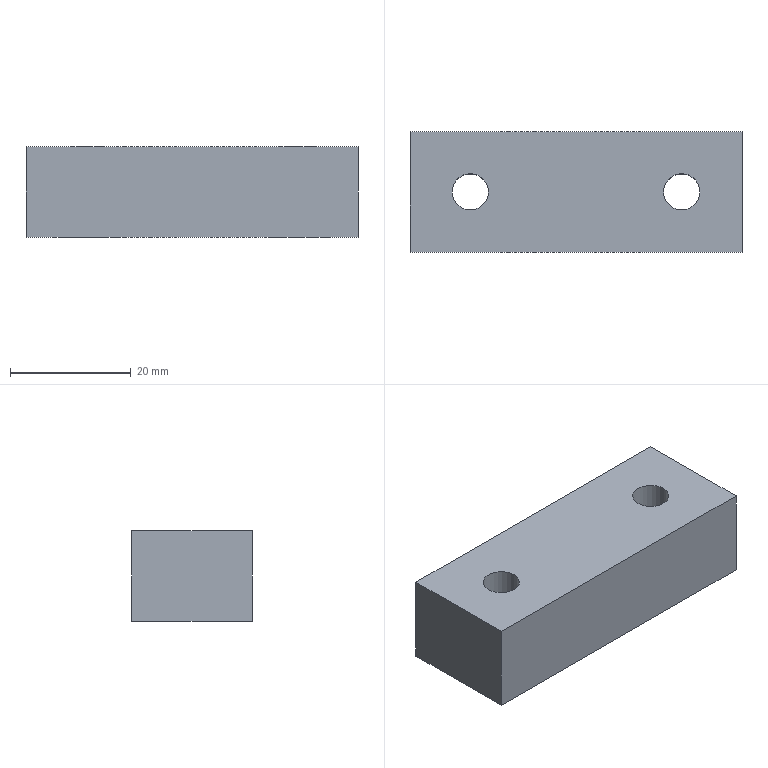Part | STEP file | gslz 2016.10.28-10_id2086_x_t | 1 solid | 12 faces | box 55 x 20 x 15 mm | volume 14584 mm3 | plane 8 | cylinder 4 | commonest cylinder face diameters 6 x2 11 x2
STEP:
#1=CARTESIAN_POINT('',(0.,0.,0.));
#2=DIRECTION('',(0.,0.,1.));
#3=DIRECTION('',(1.,0.,0.));
#4=AXIS2_PLACEMENT_3D('',#1,#2,#3);
#5=CARTESIAN_POINT('',(353.5,240.,28.));
#6=VERTEX_POINT('',#5);
#7=CARTESIAN_POINT('',(359.,240.,28.));
#8=DIRECTION('',(0.,0.,1.));
#9=DIRECTION('',(-1.,0.,0.));
#10=AXIS2_PLACEMENT_3D('',#7,#8,#9);
#11=CIRCLE('',#10,5.5);
#12=CARTESIAN_POINT('',(359.,240.,30.));
#13=DIRECTION('',(0.,0.,-1.));
#14=DIRECTION('',(-1.,0.,0.));
#15=AXIS2_PLACEMENT_3D('',#12,#13,#14);
#16=CYLINDRICAL_SURFACE('',#15,5.5);
#17=CARTESIAN_POINT('',(6.283,2.));
#18=DIRECTION('',(-1.,0.));
#19=VECTOR('',#18,1.);
#20=LINE('',#17,#19);
#21=(GEOMETRIC_REPRESENTATION_CONTEXT(2)PARAMETRIC_REPRESENTATION_CONTEXT()REPRESENTATION_CONTEXT('',''));
#22=DEFINITIONAL_REPRESENTATION('',(#20),#21);
#23=PCURVE('',#16,#22);
#24=CARTESIAN_POINT('',(396.5,240.,28.));
#25=DIRECTION('',(0.,0.,-1.));
#26=DIRECTION('',(1.,0.,0.));
#27=AXIS2_PLACEMENT_3D('',#24,#25,#26);
#28=PLANE('',#27);
#29=CARTESIAN_POINT('',(-43.,0.));
#30=CARTESIAN_POINT('',(-43.,9.526));
#31=CARTESIAN_POINT('',(-34.75,4.763));
#32=CARTESIAN_POINT('',(-26.5,0.));
#33=CARTESIAN_POINT('',(-34.75,-4.763));
#34=CARTESIAN_POINT('',(-43.,-9.526));
#35=CARTESIAN_POINT('',(-43.,0.));
#36=(BOUNDED_CURVE()B_SPLINE_CURVE(2,(#29,#30,#31,#32,#33,#34,#35),.UNSPECIFIED.,.T.,.F.)B_SPLINE_CURVE_WITH_KNOTS((1,2,2,2,2,1),(-2.094,0.,2.094,4.189,6.283,8.378),.UNSPECIFIED.)CURVE()GEOMETRIC_REPRESENTATION_ITEM()RATIONAL_B_SPLINE_CURVE((1.,0.5,1.,0.5,1.,0.5,1.))REPRESENTATION_ITEM(''));
#37=(GEOMETRIC_REPRESENTATION_CONTEXT(2)PARAMETRIC_REPRESENTATION_CONTEXT()REPRESENTATION_CONTEXT('',''));
#38=DEFINITIONAL_REPRESENTATION('',(#36),#37);
#39=PCURVE('',#28,#38);
#40=SURFACE_CURVE('',#11,(#23,#39),.PCURVE_S1.);
#41=EDGE_CURVE('',#6,#6,#40,.T.);
#42=ORIENTED_EDGE('',*,*,#41,.F.);
#43=CARTESIAN_POINT('',(353.5,240.,20.));
#44=VERTEX_POINT('',#43);
#45=CARTESIAN_POINT('',(353.5,240.,28.));
#46=CARTESIAN_POINT('',(353.5,240.,20.));
#47=B_SPLINE_CURVE_WITH_KNOTS('',1,(#45,#46),.UNSPECIFIED.,.F.,.F.,(2,2),(2.,10.),.PIECEWISE_BEZIER_KNOTS.);
#48=CARTESIAN_POINT('',(6.283,0.));
#49=DIRECTION('',(0.,1.));
#50=VECTOR('',#49,1.);
#51=LINE('',#48,#50);
#52=(GEOMETRIC_REPRESENTATION_CONTEXT(2)PARAMETRIC_REPRESENTATION_CONTEXT()REPRESENTATION_CONTEXT('',''));
#53=DEFINITIONAL_REPRESENTATION('',(#51),#52);
#54=PCURVE('',#16,#53);
#55=CARTESIAN_POINT('',(0.,0.));
#56=DIRECTION('',(0.,1.));
#57=VECTOR('',#56,1.);
#58=LINE('',#55,#57);
#59=(GEOMETRIC_REPRESENTATION_CONTEXT(2)PARAMETRIC_REPRESENTATION_CONTEXT()REPRESENTATION_CONTEXT('',''));
#60=DEFINITIONAL_REPRESENTATION('',(#58),#59);
#61=PCURVE('',#16,#60);
#62=SEAM_CURVE('',#47,(#54,#61),.PCURVE_S1.);
#63=EDGE_CURVE('',#6,#44,#62,.T.);
#64=ORIENTED_EDGE('',*,*,#63,.T.);
#65=CARTESIAN_POINT('',(364.5,240.,20.));
#66=VERTEX_POINT('',#65);
#67=CARTESIAN_POINT('',(359.,240.,20.));
#68=DIRECTION('',(0.,0.,1.));
#69=DIRECTION('',(1.,0.,0.));
#70=AXIS2_PLACEMENT_3D('',#67,#68,#69);
#71=CIRCLE('',#70,5.5);
#72=CARTESIAN_POINT('',(9.425,10.));
#73=DIRECTION('',(-1.,0.));
#74=VECTOR('',#73,1.);
#75=LINE('',#72,#74);
#76=(GEOMETRIC_REPRESENTATION_CONTEXT(2)PARAMETRIC_REPRESENTATION_CONTEXT()REPRESENTATION_CONTEXT('',''));
#77=DEFINITIONAL_REPRESENTATION('',(#75),#76);
#78=PCURVE('',#16,#77);
#79=CARTESIAN_POINT('',(301.5,240.,20.));
#80=DIRECTION('',(0.,0.,1.));
#81=DIRECTION('',(1.,0.,0.));
#82=AXIS2_PLACEMENT_3D('',#79,#80,#81);
#83=PLANE('',#82);
#84=CARTESIAN_POINT('',(57.5,0.));
#85=DIRECTION('',(1.,0.));
#86=AXIS2_PLACEMENT_2D('',#84,#85);
#87=CIRCLE('',#86,5.5);
#88=(GEOMETRIC_REPRESENTATION_CONTEXT(2)PARAMETRIC_REPRESENTATION_CONTEXT()REPRESENTATION_CONTEXT('',''));
#89=DEFINITIONAL_REPRESENTATION('',(#87),#88);
#90=PCURVE('',#83,#89);
#91=SURFACE_CURVE('',#71,(#78,#90),.PCURVE_S1.);
#92=EDGE_CURVE('',#44,#66,#91,.T.);
#93=ORIENTED_EDGE('',*,*,#92,.T.);
#94=CARTESIAN_POINT('',(359.,240.,20.));
#95=DIRECTION('',(0.,0.,1.));
#96=DIRECTION('',(1.,0.,0.));
#97=AXIS2_PLACEMENT_3D('',#94,#95,#96);
#98=CIRCLE('',#97,5.5);
#99=CARTESIAN_POINT('',(3.142,10.));
#100=DIRECTION('',(-1.,0.));
#101=VECTOR('',#100,1.);
#102=LINE('',#99,#101);
#103=(GEOMETRIC_REPRESENTATION_CONTEXT(2)PARAMETRIC_REPRESENTATION_CONTEXT()REPRESENTATION_CONTEXT('',''));
#104=DEFINITIONAL_REPRESENTATION('',(#102),#103);
#105=PCURVE('',#16,#104);
#106=CARTESIAN_POINT('',(57.5,0.));
#107=DIRECTION('',(1.,0.));
#108=AXIS2_PLACEMENT_2D('',#106,#107);
#109=CIRCLE('',#108,5.5);
#110=(GEOMETRIC_REPRESENTATION_CONTEXT(2)PARAMETRIC_REPRESENTATION_CONTEXT()REPRESENTATION_CONTEXT('',''));
#111=DEFINITIONAL_REPRESENTATION('',(#109),#110);
#112=PCURVE('',#83,#111);
#113=SURFACE_CURVE('',#98,(#105,#112),.PCURVE_S1.);
#114=EDGE_CURVE('',#66,#44,#113,.T.);
#115=ORIENTED_EDGE('',*,*,#114,.T.);
#116=ORIENTED_EDGE('',*,*,#63,.F.);
#117=EDGE_LOOP('',(#42,#64,#93,#115,#116));
#118=FACE_BOUND('',#117,.F.);
#119=ADVANCED_FACE('',(#118),#16,.F.);
#120=CARTESIAN_POINT('',(349.,250.,35.));
#121=VERTEX_POINT('',#120);
#122=CARTESIAN_POINT('',(349.,250.,20.));
#123=VERTEX_POINT('',#122);
#124=CARTESIAN_POINT('',(349.,250.,30.));
#125=DIRECTION('',(0.,0.,-1.));
#126=VECTOR('',#125,1.);
#127=LINE('',#124,#126);
#128=CARTESIAN_POINT('',(421.5,250.,30.));
#129=DIRECTION('',(0.,-1.,0.));
#130=DIRECTION('',(0.,0.,-1.));
#131=AXIS2_PLACEMENT_3D('',#128,#129,#130);
#132=PLANE('',#131);
#133=CARTESIAN_POINT('',(0.,-72.5));
#134=DIRECTION('',(1.,0.));
#135=VECTOR('',#134,1.);
#136=LINE('',#133,#135);
#137=(GEOMETRIC_REPRESENTATION_CONTEXT(2)PARAMETRIC_REPRESENTATION_CONTEXT()REPRESENTATION_CONTEXT('',''));
#138=DEFINITIONAL_REPRESENTATION('',(#136),#137);
#139=PCURVE('',#132,#138);
#140=CARTESIAN_POINT('',(349.,252.5,30.));
#141=DIRECTION('',(1.,0.,0.));
#142=DIRECTION('',(0.,0.,-1.));
#143=AXIS2_PLACEMENT_3D('',#140,#141,#142);
#144=PLANE('',#143);
#145=CARTESIAN_POINT('',(0.,-2.5));
#146=DIRECTION('',(1.,0.));
#147=VECTOR('',#146,1.);
#148=LINE('',#145,#147);
#149=(GEOMETRIC_REPRESENTATION_CONTEXT(2)PARAMETRIC_REPRESENTATION_CONTEXT()REPRESENTATION_CONTEXT('',''));
#150=DEFINITIONAL_REPRESENTATION('',(#148),#149);
#151=PCURVE('',#144,#150);
#152=SURFACE_CURVE('',#127,(#139,#151),.PCURVE_S1.);
#153=EDGE_CURVE('',#121,#123,#152,.T.);
#154=ORIENTED_EDGE('',*,*,#153,.F.);
#155=CARTESIAN_POINT('',(404.,250.,35.));
#156=VERTEX_POINT('',#155);
#157=CARTESIAN_POINT('',(301.5,250.,35.));
#158=DIRECTION('',(-1.,0.,0.));
#159=VECTOR('',#158,1.);
#160=LINE('',#157,#159);
#161=CARTESIAN_POINT('',(-5.,-120.));
#162=DIRECTION('',(0.,-1.));
#163=VECTOR('',#162,1.);
#164=LINE('',#161,#163);
#165=(GEOMETRIC_REPRESENTATION_CONTEXT(2)PARAMETRIC_REPRESENTATION_CONTEXT()REPRESENTATION_CONTEXT('',''));
#166=DEFINITIONAL_REPRESENTATION('',(#164),#165);
#167=PCURVE('',#132,#166);
#168=CARTESIAN_POINT('',(301.5,240.,35.));
#169=DIRECTION('',(0.,0.,1.));
#170=DIRECTION('',(1.,0.,0.));
#171=AXIS2_PLACEMENT_3D('',#168,#169,#170);
#172=PLANE('',#171);
#173=CARTESIAN_POINT('',(0.,10.));
#174=DIRECTION('',(-1.,0.));
#175=VECTOR('',#174,1.);
#176=LINE('',#173,#175);
#177=(GEOMETRIC_REPRESENTATION_CONTEXT(2)PARAMETRIC_REPRESENTATION_CONTEXT()REPRESENTATION_CONTEXT('',''));
#178=DEFINITIONAL_REPRESENTATION('',(#176),#177);
#179=PCURVE('',#172,#178);
#180=SURFACE_CURVE('',#160,(#167,#179),.PCURVE_S1.);
#181=EDGE_CURVE('',#156,#121,#180,.T.);
#182=ORIENTED_EDGE('',*,*,#181,.F.);
#183=CARTESIAN_POINT('',(404.,250.,20.));
#184=VERTEX_POINT('',#183);
#185=CARTESIAN_POINT('',(404.,250.,30.));
#186=DIRECTION('',(0.,0.,-1.));
#187=VECTOR('',#186,1.);
#188=LINE('',#185,#187);
#189=CARTESIAN_POINT('',(0.,-17.5));
#190=DIRECTION('',(1.,0.));
#191=VECTOR('',#190,1.);
#192=LINE('',#189,#191);
#193=(GEOMETRIC_REPRESENTATION_CONTEXT(2)PARAMETRIC_REPRESENTATION_CONTEXT()REPRESENTATION_CONTEXT('',''));
#194=DEFINITIONAL_REPRESENTATION('',(#192),#193);
#195=PCURVE('',#132,#194);
#196=CARTESIAN_POINT('',(404.,227.5,30.));
#197=DIRECTION('',(-1.,0.,0.));
#198=DIRECTION('',(0.,0.,1.));
#199=AXIS2_PLACEMENT_3D('',#196,#197,#198);
#200=PLANE('',#199);
#201=CARTESIAN_POINT('',(0.,22.5));
#202=DIRECTION('',(-1.,0.));
#203=VECTOR('',#202,1.);
#204=LINE('',#201,#203);
#205=(GEOMETRIC_REPRESENTATION_CONTEXT(2)PARAMETRIC_REPRESENTATION_CONTEXT()REPRESENTATION_CONTEXT('',''));
#206=DEFINITIONAL_REPRESENTATION('',(#204),#205);
#207=PCURVE('',#200,#206);
#208=SURFACE_CURVE('',#188,(#195,#207),.PCURVE_S1.);
#209=EDGE_CURVE('',#156,#184,#208,.T.);
#210=ORIENTED_EDGE('',*,*,#209,.T.);
#211=CARTESIAN_POINT('',(301.5,250.,20.));
#212=DIRECTION('',(-1.,0.,0.));
#213=VECTOR('',#212,1.);
#214=LINE('',#211,#213);
#215=CARTESIAN_POINT('',(10.,-120.));
#216=DIRECTION('',(0.,-1.));
#217=VECTOR('',#216,1.);
#218=LINE('',#215,#217);
#219=(GEOMETRIC_REPRESENTATION_CONTEXT(2)PARAMETRIC_REPRESENTATION_CONTEXT()REPRESENTATION_CONTEXT('',''));
#220=DEFINITIONAL_REPRESENTATION('',(#218),#219);
#221=PCURVE('',#132,#220);
#222=CARTESIAN_POINT('',(0.,10.));
#223=DIRECTION('',(-1.,0.));
#224=VECTOR('',#223,1.);
#225=LINE('',#222,#224);
#226=(GEOMETRIC_REPRESENTATION_CONTEXT(2)PARAMETRIC_REPRESENTATION_CONTEXT()REPRESENTATION_CONTEXT('',''));
#227=DEFINITIONAL_REPRESENTATION('',(#225),#226);
#228=PCURVE('',#83,#227);
#229=SURFACE_CURVE('',#214,(#221,#228),.PCURVE_S1.);
#230=EDGE_CURVE('',#184,#123,#229,.T.);
#231=ORIENTED_EDGE('',*,*,#230,.T.);
#232=EDGE_LOOP('',(#154,#182,#210,#231));
#233=FACE_BOUND('',#232,.T.);
#234=ADVANCED_FACE('',(#233),#132,.F.);
#235=ORIENTED_EDGE('',*,*,#209,.F.);
#236=CARTESIAN_POINT('',(404.,230.,35.));
#237=VERTEX_POINT('',#236);
#238=CARTESIAN_POINT('',(404.,227.5,35.));
#239=DIRECTION('',(0.,1.,0.));
#240=VECTOR('',#239,1.);
#241=LINE('',#238,#240);
#242=CARTESIAN_POINT('',(5.,0.));
#243=DIRECTION('',(0.,1.));
#244=VECTOR('',#243,1.);
#245=LINE('',#242,#244);
#246=(GEOMETRIC_REPRESENTATION_CONTEXT(2)PARAMETRIC_REPRESENTATION_CONTEXT()REPRESENTATION_CONTEXT('',''));
#247=DEFINITIONAL_REPRESENTATION('',(#245),#246);
#248=PCURVE('',#200,#247);
#249=CARTESIAN_POINT('',(102.5,-12.5));
#250=DIRECTION('',(0.,1.));
#251=VECTOR('',#250,1.);
#252=LINE('',#249,#251);
#253=(GEOMETRIC_REPRESENTATION_CONTEXT(2)PARAMETRIC_REPRESENTATION_CONTEXT()REPRESENTATION_CONTEXT('',''));
#254=DEFINITIONAL_REPRESENTATION('',(#252),#253);
#255=PCURVE('',#172,#254);
#256=SURFACE_CURVE('',#241,(#248,#255),.PCURVE_S1.);
#257=EDGE_CURVE('',#237,#156,#256,.T.);
#258=ORIENTED_EDGE('',*,*,#257,.F.);
#259=CARTESIAN_POINT('',(404.,230.,20.));
#260=VERTEX_POINT('',#259);
#261=CARTESIAN_POINT('',(404.,230.,30.));
#262=DIRECTION('',(0.,0.,-1.));
#263=VECTOR('',#262,1.);
#264=LINE('',#261,#263);
#265=CARTESIAN_POINT('',(0.,2.5));
#266=DIRECTION('',(-1.,0.));
#267=VECTOR('',#266,1.);
#268=LINE('',#265,#267);
#269=(GEOMETRIC_REPRESENTATION_CONTEXT(2)PARAMETRIC_REPRESENTATION_CONTEXT()REPRESENTATION_CONTEXT('',''));
#270=DEFINITIONAL_REPRESENTATION('',(#268),#269);
#271=PCURVE('',#200,#270);
#272=CARTESIAN_POINT('',(291.5,230.,30.));
#273=DIRECTION('',(0.,1.,0.));
#274=DIRECTION('',(0.,0.,1.));
#275=AXIS2_PLACEMENT_3D('',#272,#273,#274);
#276=PLANE('',#275);
#277=CARTESIAN_POINT('',(0.,112.5));
#278=DIRECTION('',(-1.,0.));
#279=VECTOR('',#278,1.);
#280=LINE('',#277,#279);
#281=(GEOMETRIC_REPRESENTATION_CONTEXT(2)PARAMETRIC_REPRESENTATION_CONTEXT()REPRESENTATION_CONTEXT('',''));
#282=DEFINITIONAL_REPRESENTATION('',(#280),#281);
#283=PCURVE('',#276,#282);
#284=SURFACE_CURVE('',#264,(#271,#283),.PCURVE_S1.);
#285=EDGE_CURVE('',#237,#260,#284,.T.);
#286=ORIENTED_EDGE('',*,*,#285,.T.);
#287=CARTESIAN_POINT('',(404.,227.5,20.));
#288=DIRECTION('',(0.,1.,0.));
#289=VECTOR('',#288,1.);
#290=LINE('',#287,#289);
#291=CARTESIAN_POINT('',(-10.,0.));
#292=DIRECTION('',(0.,1.));
#293=VECTOR('',#292,1.);
#294=LINE('',#291,#293);
#295=(GEOMETRIC_REPRESENTATION_CONTEXT(2)PARAMETRIC_REPRESENTATION_CONTEXT()REPRESENTATION_CONTEXT('',''));
#296=DEFINITIONAL_REPRESENTATION('',(#294),#295);
#297=PCURVE('',#200,#296);
#298=CARTESIAN_POINT('',(102.5,-12.5));
#299=DIRECTION('',(0.,1.));
#300=VECTOR('',#299,1.);
#301=LINE('',#298,#300);
#302=(GEOMETRIC_REPRESENTATION_CONTEXT(2)PARAMETRIC_REPRESENTATION_CONTEXT()REPRESENTATION_CONTEXT('',''));
#303=DEFINITIONAL_REPRESENTATION('',(#301),#302);
#304=PCURVE('',#83,#303);
#305=SURFACE_CURVE('',#290,(#297,#304),.PCURVE_S1.);
#306=EDGE_CURVE('',#260,#184,#305,.T.);
#307=ORIENTED_EDGE('',*,*,#306,.T.);
#308=EDGE_LOOP('',(#235,#258,#286,#307));
#309=FACE_BOUND('',#308,.T.);
#310=ADVANCED_FACE('',(#309),#200,.F.);
#311=ORIENTED_EDGE('',*,*,#285,.F.);
#312=CARTESIAN_POINT('',(349.,230.,35.));
#313=VERTEX_POINT('',#312);
#314=CARTESIAN_POINT('',(301.5,230.,35.));
#315=DIRECTION('',(1.,0.,0.));
#316=VECTOR('',#315,1.);
#317=LINE('',#314,#316);
#318=CARTESIAN_POINT('',(5.,10.));
#319=DIRECTION('',(0.,1.));
#320=VECTOR('',#319,1.);
#321=LINE('',#318,#320);
#322=(GEOMETRIC_REPRESENTATION_CONTEXT(2)PARAMETRIC_REPRESENTATION_CONTEXT()REPRESENTATION_CONTEXT('',''));
#323=DEFINITIONAL_REPRESENTATION('',(#321),#322);
#324=PCURVE('',#276,#323);
#325=CARTESIAN_POINT('',(0.,-10.));
#326=DIRECTION('',(1.,0.));
#327=VECTOR('',#326,1.);
#328=LINE('',#325,#327);
#329=(GEOMETRIC_REPRESENTATION_CONTEXT(2)PARAMETRIC_REPRESENTATION_CONTEXT()REPRESENTATION_CONTEXT('',''));
#330=DEFINITIONAL_REPRESENTATION('',(#328),#329);
#331=PCURVE('',#172,#330);
#332=SURFACE_CURVE('',#317,(#324,#331),.PCURVE_S1.);
#333=EDGE_CURVE('',#313,#237,#332,.T.);
#334=ORIENTED_EDGE('',*,*,#333,.F.);
#335=CARTESIAN_POINT('',(349.,230.,20.));
#336=VERTEX_POINT('',#335);
#337=CARTESIAN_POINT('',(349.,230.,30.));
#338=DIRECTION('',(0.,0.,-1.));
#339=VECTOR('',#338,1.);
#340=LINE('',#337,#339);
#341=CARTESIAN_POINT('',(0.,57.5));
#342=DIRECTION('',(-1.,0.));
#343=VECTOR('',#342,1.);
#344=LINE('',#341,#343);
#345=(GEOMETRIC_REPRESENTATION_CONTEXT(2)PARAMETRIC_REPRESENTATION_CONTEXT()REPRESENTATION_CONTEXT('',''));
#346=DEFINITIONAL_REPRESENTATION('',(#344),#345);
#347=PCURVE('',#276,#346);
#348=CARTESIAN_POINT('',(0.,-22.5));
#349=DIRECTION('',(1.,0.));
#350=VECTOR('',#349,1.);
#351=LINE('',#348,#350);
#352=(GEOMETRIC_REPRESENTATION_CONTEXT(2)PARAMETRIC_REPRESENTATION_CONTEXT()REPRESENTATION_CONTEXT('',''));
#353=DEFINITIONAL_REPRESENTATION('',(#351),#352);
#354=PCURVE('',#144,#353);
#355=SURFACE_CURVE('',#340,(#347,#354),.PCURVE_S1.);
#356=EDGE_CURVE('',#313,#336,#355,.T.);
#357=ORIENTED_EDGE('',*,*,#356,.T.);
#358=CARTESIAN_POINT('',(301.5,230.,20.));
#359=DIRECTION('',(1.,0.,0.));
#360=VECTOR('',#359,1.);
#361=LINE('',#358,#360);
#362=CARTESIAN_POINT('',(-10.,10.));
#363=DIRECTION('',(0.,1.));
#364=VECTOR('',#363,1.);
#365=LINE('',#362,#364);
#366=(GEOMETRIC_REPRESENTATION_CONTEXT(2)PARAMETRIC_REPRESENTATION_CONTEXT()REPRESENTATION_CONTEXT('',''));
#367=DEFINITIONAL_REPRESENTATION('',(#365),#366);
#368=PCURVE('',#276,#367);
#369=CARTESIAN_POINT('',(0.,-10.));
#370=DIRECTION('',(1.,0.));
#371=VECTOR('',#370,1.);
#372=LINE('',#369,#371);
#373=(GEOMETRIC_REPRESENTATION_CONTEXT(2)PARAMETRIC_REPRESENTATION_CONTEXT()REPRESENTATION_CONTEXT('',''));
#374=DEFINITIONAL_REPRESENTATION('',(#372),#373);
#375=PCURVE('',#83,#374);
#376=SURFACE_CURVE('',#361,(#368,#375),.PCURVE_S1.);
#377=EDGE_CURVE('',#336,#260,#376,.T.);
#378=ORIENTED_EDGE('',*,*,#377,.T.);
#379=EDGE_LOOP('',(#311,#334,#357,#378));
#380=FACE_BOUND('',#379,.T.);
#381=ADVANCED_FACE('',(#380),#276,.F.);
#382=ORIENTED_EDGE('',*,*,#356,.F.);
#383=CARTESIAN_POINT('',(349.,252.5,35.));
#384=DIRECTION('',(0.,-1.,0.));
#385=VECTOR('',#384,1.);
#386=LINE('',#383,#385);
#387=CARTESIAN_POINT('',(-5.,0.));
#388=DIRECTION('',(0.,-1.));
#389=VECTOR('',#388,1.);
#390=LINE('',#387,#389);
#391=(GEOMETRIC_REPRESENTATION_CONTEXT(2)PARAMETRIC_REPRESENTATION_CONTEXT()REPRESENTATION_CONTEXT('',''));
#392=DEFINITIONAL_REPRESENTATION('',(#390),#391);
#393=PCURVE('',#144,#392);
#394=CARTESIAN_POINT('',(47.5,12.5));
#395=DIRECTION('',(0.,-1.));
#396=VECTOR('',#395,1.);
#397=LINE('',#394,#396);
#398=(GEOMETRIC_REPRESENTATION_CONTEXT(2)PARAMETRIC_REPRESENTATION_CONTEXT()REPRESENTATION_CONTEXT('',''));
#399=DEFINITIONAL_REPRESENTATION('',(#397),#398);
#400=PCURVE('',#172,#399);
#401=SURFACE_CURVE('',#386,(#393,#400),.PCURVE_S1.);
#402=EDGE_CURVE('',#121,#313,#401,.T.);
#403=ORIENTED_EDGE('',*,*,#402,.F.);
#404=ORIENTED_EDGE('',*,*,#153,.T.);
#405=CARTESIAN_POINT('',(349.,252.5,20.));
#406=DIRECTION('',(0.,-1.,0.));
#407=VECTOR('',#406,1.);
#408=LINE('',#405,#407);
#409=CARTESIAN_POINT('',(10.,0.));
#410=DIRECTION('',(0.,-1.));
#411=VECTOR('',#410,1.);
#412=LINE('',#409,#411);
#413=(GEOMETRIC_REPRESENTATION_CONTEXT(2)PARAMETRIC_REPRESENTATION_CONTEXT()REPRESENTATION_CONTEXT('',''));
#414=DEFINITIONAL_REPRESENTATION('',(#412),#413);
#415=PCURVE('',#144,#414);
#416=CARTESIAN_POINT('',(47.5,12.5));
#417=DIRECTION('',(0.,-1.));
#418=VECTOR('',#417,1.);
#419=LINE('',#416,#418);
#420=(GEOMETRIC_REPRESENTATION_CONTEXT(2)PARAMETRIC_REPRESENTATION_CONTEXT()REPRESENTATION_CONTEXT('',''));
#421=DEFINITIONAL_REPRESENTATION('',(#419),#420);
#422=PCURVE('',#83,#421);
#423=SURFACE_CURVE('',#408,(#415,#422),.PCURVE_S1.);
#424=EDGE_CURVE('',#123,#336,#423,.T.);
#425=ORIENTED_EDGE('',*,*,#424,.T.);
#426=EDGE_LOOP('',(#382,#403,#404,#425));
#427=FACE_BOUND('',#426,.T.);
#428=ADVANCED_FACE('',(#427),#144,.F.);
#429=ORIENTED_EDGE('',*,*,#424,.F.);
#430=ORIENTED_EDGE('',*,*,#230,.F.);
#431=ORIENTED_EDGE('',*,*,#306,.F.);
#432=ORIENTED_EDGE('',*,*,#377,.F.);
#433=EDGE_LOOP('',(#429,#430,#431,#432));
#434=FACE_BOUND('',#433,.T.);
#435=ORIENTED_EDGE('',*,*,#114,.T.);
#436=ORIENTED_EDGE('',*,*,#92,.T.);
#437=EDGE_LOOP('',(#435,#436));
#438=FACE_BOUND('',#437,.T.);
#439=CARTESIAN_POINT('',(399.5,240.,20.));
#440=VERTEX_POINT('',#439);
#441=CARTESIAN_POINT('',(388.5,240.,20.));
#442=VERTEX_POINT('',#441);
#443=CARTESIAN_POINT('',(394.,240.,20.));
#444=DIRECTION('',(0.,0.,1.));
#445=DIRECTION('',(1.,0.,0.));
#446=AXIS2_PLACEMENT_3D('',#443,#444,#445);
#447=CIRCLE('',#446,5.5);
#448=CARTESIAN_POINT('',(92.5,0.));
#449=DIRECTION('',(1.,0.));
#450=AXIS2_PLACEMENT_2D('',#448,#449);
#451=CIRCLE('',#450,5.5);
#452=(GEOMETRIC_REPRESENTATION_CONTEXT(2)PARAMETRIC_REPRESENTATION_CONTEXT()REPRESENTATION_CONTEXT('',''));
#453=DEFINITIONAL_REPRESENTATION('',(#451),#452);
#454=PCURVE('',#83,#453);
#455=CARTESIAN_POINT('',(394.,240.,30.));
#456=DIRECTION('',(0.,0.,-1.));
#457=DIRECTION('',(-1.,0.,0.));
#458=AXIS2_PLACEMENT_3D('',#455,#456,#457);
#459=CYLINDRICAL_SURFACE('',#458,5.5);
#460=CARTESIAN_POINT('',(3.142,10.));
#461=DIRECTION('',(-1.,0.));
#462=VECTOR('',#461,1.);
#463=LINE('',#460,#462);
#464=(GEOMETRIC_REPRESENTATION_CONTEXT(2)PARAMETRIC_REPRESENTATION_CONTEXT()REPRESENTATION_CONTEXT('',''));
#465=DEFINITIONAL_REPRESENTATION('',(#463),#464);
#466=PCURVE('',#459,#465);
#467=SURFACE_CURVE('',#447,(#454,#466),.PCURVE_S1.);
#468=EDGE_CURVE('',#440,#442,#467,.T.);
#469=ORIENTED_EDGE('',*,*,#468,.T.);
#470=CARTESIAN_POINT('',(394.,240.,20.));
#471=DIRECTION('',(0.,0.,1.));
#472=DIRECTION('',(1.,0.,0.));
#473=AXIS2_PLACEMENT_3D('',#470,#471,#472);
#474=CIRCLE('',#473,5.5);
#475=CARTESIAN_POINT('',(92.5,0.));
#476=DIRECTION('',(1.,0.));
#477=AXIS2_PLACEMENT_2D('',#475,#476);
#478=CIRCLE('',#477,5.5);
#479=(GEOMETRIC_REPRESENTATION_CONTEXT(2)PARAMETRIC_REPRESENTATION_CONTEXT()REPRESENTATION_CONTEXT('',''));
#480=DEFINITIONAL_REPRESENTATION('',(#478),#479);
#481=PCURVE('',#83,#480);
#482=CARTESIAN_POINT('',(9.425,10.));
#483=DIRECTION('',(-1.,0.));
#484=VECTOR('',#483,1.);
#485=LINE('',#482,#484);
#486=(GEOMETRIC_REPRESENTATION_CONTEXT(2)PARAMETRIC_REPRESENTATION_CONTEXT()REPRESENTATION_CONTEXT('',''));
#487=DEFINITIONAL_REPRESENTATION('',(#485),#486);
#488=PCURVE('',#459,#487);
#489=SURFACE_CURVE('',#474,(#481,#488),.PCURVE_S1.);
#490=EDGE_CURVE('',#442,#440,#489,.T.);
#491=ORIENTED_EDGE('',*,*,#490,.T.);
#492=EDGE_LOOP('',(#469,#491));
#493=FACE_BOUND('',#492,.T.);
#494=ADVANCED_FACE('',(#434,#438,#493),#83,.F.);
#495=CARTESIAN_POINT('',(388.5,240.,28.));
#496=VERTEX_POINT('',#495);
#497=CARTESIAN_POINT('',(394.,240.,28.));
#498=DIRECTION('',(0.,0.,1.));
#499=DIRECTION('',(-1.,0.,0.));
#500=AXIS2_PLACEMENT_3D('',#497,#498,#499);
#501=CIRCLE('',#500,5.5);
#502=CARTESIAN_POINT('',(6.283,2.));
#503=DIRECTION('',(-1.,0.));
#504=VECTOR('',#503,1.);
#505=LINE('',#502,#504);
#506=(GEOMETRIC_REPRESENTATION_CONTEXT(2)PARAMETRIC_REPRESENTATION_CONTEXT()REPRESENTATION_CONTEXT('',''));
#507=DEFINITIONAL_REPRESENTATION('',(#505),#506);
#508=PCURVE('',#459,#507);
#509=CARTESIAN_POINT('',(356.5,240.,28.));
#510=DIRECTION('',(0.,0.,-1.));
#511=DIRECTION('',(1.,0.,0.));
#512=AXIS2_PLACEMENT_3D('',#509,#510,#511);
#513=PLANE('',#512);
#514=CARTESIAN_POINT('',(32.,0.));
#515=CARTESIAN_POINT('',(32.,9.526));
#516=CARTESIAN_POINT('',(40.25,4.763));
#517=CARTESIAN_POINT('',(48.5,0.));
#518=CARTESIAN_POINT('',(40.25,-4.763));
#519=CARTESIAN_POINT('',(32.,-9.526));
#520=CARTESIAN_POINT('',(32.,0.));
#521=(BOUNDED_CURVE()B_SPLINE_CURVE(2,(#514,#515,#516,#517,#518,#519,#520),.UNSPECIFIED.,.T.,.F.)B_SPLINE_CURVE_WITH_KNOTS((1,2,2,2,2,1),(-2.094,0.,2.094,4.189,6.283,8.378),.UNSPECIFIED.)CURVE()GEOMETRIC_REPRESENTATION_ITEM()RATIONAL_B_SPLINE_CURVE((1.,0.5,1.,0.5,1.,0.5,1.))REPRESENTATION_ITEM(''));
#522=(GEOMETRIC_REPRESENTATION_CONTEXT(2)PARAMETRIC_REPRESENTATION_CONTEXT()REPRESENTATION_CONTEXT('',''));
#523=DEFINITIONAL_REPRESENTATION('',(#521),#522);
#524=PCURVE('',#513,#523);
#525=SURFACE_CURVE('',#501,(#508,#524),.PCURVE_S1.);
#526=EDGE_CURVE('',#496,#496,#525,.T.);
#527=ORIENTED_EDGE('',*,*,#526,.F.);
#528=CARTESIAN_POINT('',(388.5,240.,28.));
#529=CARTESIAN_POINT('',(388.5,240.,20.));
#530=B_SPLINE_CURVE_WITH_KNOTS('',1,(#528,#529),.UNSPECIFIED.,.F.,.F.,(2,2),(2.,10.),.PIECEWISE_BEZIER_KNOTS.);
#531=CARTESIAN_POINT('',(6.283,0.));
#532=DIRECTION('',(0.,1.));
#533=VECTOR('',#532,1.);
#534=LINE('',#531,#533);
#535=(GEOMETRIC_REPRESENTATION_CONTEXT(2)PARAMETRIC_REPRESENTATION_CONTEXT()REPRESENTATION_CONTEXT('',''));
#536=DEFINITIONAL_REPRESENTATION('',(#534),#535);
#537=PCURVE('',#459,#536);
#538=CARTESIAN_POINT('',(0.,0.));
#539=DIRECTION('',(0.,1.));
#540=VECTOR('',#539,1.);
#541=LINE('',#538,#540);
#542=(GEOMETRIC_REPRESENTATION_CONTEXT(2)PARAMETRIC_REPRESENTATION_CONTEXT()REPRESENTATION_CONTEXT('',''));
#543=DEFINITIONAL_REPRESENTATION('',(#541),#542);
#544=PCURVE('',#459,#543);
#545=SEAM_CURVE('',#530,(#537,#544),.PCURVE_S1.);
#546=EDGE_CURVE('',#496,#442,#545,.T.);
#547=ORIENTED_EDGE('',*,*,#546,.T.);
#548=ORIENTED_EDGE('',*,*,#490,.T.);
#549=ORIENTED_EDGE('',*,*,#468,.T.);
#550=ORIENTED_EDGE('',*,*,#546,.F.);
#551=EDGE_LOOP('',(#527,#547,#548,#549,#550));
#552=FACE_BOUND('',#551,.F.);
#553=ADVANCED_FACE('',(#552),#459,.F.);
#554=CARTESIAN_POINT('',(391.,240.,28.));
#555=VERTEX_POINT('',#554);
#556=CARTESIAN_POINT('',(394.,240.,28.));
#557=DIRECTION('',(0.,0.,-1.));
#558=DIRECTION('',(-1.,0.,0.));
#559=AXIS2_PLACEMENT_3D('',#556,#557,#558);
#560=CIRCLE('',#559,3.);
#561=CARTESIAN_POINT('',(37.5,0.));
#562=DIRECTION('',(-1.,0.));
#563=AXIS2_PLACEMENT_2D('',#561,#562);
#564=CIRCLE('',#563,3.);
#565=(GEOMETRIC_REPRESENTATION_CONTEXT(2)PARAMETRIC_REPRESENTATION_CONTEXT()REPRESENTATION_CONTEXT('',''));
#566=DEFINITIONAL_REPRESENTATION('',(#564),#565);
#567=PCURVE('',#513,#566);
#568=CARTESIAN_POINT('',(394.,240.,30.));
#569=DIRECTION('',(0.,0.,-1.));
#570=DIRECTION('',(-1.,0.,0.));
#571=AXIS2_PLACEMENT_3D('',#568,#569,#570);
#572=CYLINDRICAL_SURFACE('',#571,3.);
#573=CARTESIAN_POINT('',(0.,2.));
#574=DIRECTION('',(1.,0.));
#575=VECTOR('',#574,1.);
#576=LINE('',#573,#575);
#577=(GEOMETRIC_REPRESENTATION_CONTEXT(2)PARAMETRIC_REPRESENTATION_CONTEXT()REPRESENTATION_CONTEXT('',''));
#578=DEFINITIONAL_REPRESENTATION('',(#576),#577);
#579=PCURVE('',#572,#578);
#580=SURFACE_CURVE('',#560,(#567,#579),.PCURVE_S1.);
#581=EDGE_CURVE('',#555,#555,#580,.T.);
#582=ORIENTED_EDGE('',*,*,#581,.F.);
#583=EDGE_LOOP('',(#582));
#584=FACE_BOUND('',#583,.T.);
#585=ORIENTED_EDGE('',*,*,#526,.F.);
#586=EDGE_LOOP('',(#585));
#587=FACE_BOUND('',#586,.T.);
#588=ADVANCED_FACE('',(#584,#587),#513,.T.);
#589=CARTESIAN_POINT('',(356.,240.,28.));
#590=VERTEX_POINT('',#589);
#591=CARTESIAN_POINT('',(359.,240.,28.));
#592=DIRECTION('',(0.,0.,-1.));
#593=DIRECTION('',(-1.,0.,0.));
#594=AXIS2_PLACEMENT_3D('',#591,#592,#593);
#595=CIRCLE('',#594,3.);
#596=CARTESIAN_POINT('',(-37.5,0.));
#597=DIRECTION('',(-1.,0.));
#598=AXIS2_PLACEMENT_2D('',#596,#597);
#599=CIRCLE('',#598,3.);
#600=(GEOMETRIC_REPRESENTATION_CONTEXT(2)PARAMETRIC_REPRESENTATION_CONTEXT()REPRESENTATION_CONTEXT('',''));
#601=DEFINITIONAL_REPRESENTATION('',(#599),#600);
#602=PCURVE('',#28,#601);
#603=CARTESIAN_POINT('',(359.,240.,30.));
#604=DIRECTION('',(0.,0.,-1.));
#605=DIRECTION('',(-1.,0.,0.));
#606=AXIS2_PLACEMENT_3D('',#603,#604,#605);
#607=CYLINDRICAL_SURFACE('',#606,3.);
#608=CARTESIAN_POINT('',(0.,2.));
#609=DIRECTION('',(1.,0.));
#610=VECTOR('',#609,1.);
#611=LINE('',#608,#610);
#612=(GEOMETRIC_REPRESENTATION_CONTEXT(2)PARAMETRIC_REPRESENTATION_CONTEXT()REPRESENTATION_CONTEXT('',''));
#613=DEFINITIONAL_REPRESENTATION('',(#611),#612);
#614=PCURVE('',#607,#613);
#615=SURFACE_CURVE('',#595,(#602,#614),.PCURVE_S1.);
#616=EDGE_CURVE('',#590,#590,#615,.T.);
#617=ORIENTED_EDGE('',*,*,#616,.F.);
#618=EDGE_LOOP('',(#617));
#619=FACE_BOUND('',#618,.T.);
#620=ORIENTED_EDGE('',*,*,#41,.F.);
#621=EDGE_LOOP('',(#620));
#622=FACE_BOUND('',#621,.T.);
#623=ADVANCED_FACE('',(#619,#622),#28,.T.);
#624=CARTESIAN_POINT('',(356.,240.,35.));
#625=VERTEX_POINT('',#624);
#626=CARTESIAN_POINT('',(362.,240.,35.));
#627=VERTEX_POINT('',#626);
#628=CARTESIAN_POINT('',(359.,240.,35.));
#629=DIRECTION('',(0.,0.,1.));
#630=DIRECTION('',(1.,0.,0.));
#631=AXIS2_PLACEMENT_3D('',#628,#629,#630);
#632=CIRCLE('',#631,3.);
#633=CARTESIAN_POINT('',(9.425,-5.));
#634=DIRECTION('',(-1.,0.));
#635=VECTOR('',#634,1.);
#636=LINE('',#633,#635);
#637=(GEOMETRIC_REPRESENTATION_CONTEXT(2)PARAMETRIC_REPRESENTATION_CONTEXT()REPRESENTATION_CONTEXT('',''));
#638=DEFINITIONAL_REPRESENTATION('',(#636),#637);
#639=PCURVE('',#607,#638);
#640=CARTESIAN_POINT('',(57.5,0.));
#641=DIRECTION('',(1.,0.));
#642=AXIS2_PLACEMENT_2D('',#640,#641);
#643=CIRCLE('',#642,3.);
#644=(GEOMETRIC_REPRESENTATION_CONTEXT(2)PARAMETRIC_REPRESENTATION_CONTEXT()REPRESENTATION_CONTEXT('',''));
#645=DEFINITIONAL_REPRESENTATION('',(#643),#644);
#646=PCURVE('',#172,#645);
#647=SURFACE_CURVE('',#632,(#639,#646),.PCURVE_S1.);
#648=EDGE_CURVE('',#625,#627,#647,.T.);
#649=ORIENTED_EDGE('',*,*,#648,.F.);
#650=CARTESIAN_POINT('',(356.,240.,35.));
#651=CARTESIAN_POINT('',(356.,240.,28.));
#652=B_SPLINE_CURVE_WITH_KNOTS('',1,(#650,#651),.UNSPECIFIED.,.F.,.F.,(2,2),(-5.,2.),.PIECEWISE_BEZIER_KNOTS.);
#653=CARTESIAN_POINT('',(6.283,0.));
#654=DIRECTION('',(0.,1.));
#655=VECTOR('',#654,1.);
#656=LINE('',#653,#655);
#657=(GEOMETRIC_REPRESENTATION_CONTEXT(2)PARAMETRIC_REPRESENTATION_CONTEXT()REPRESENTATION_CONTEXT('',''));
#658=DEFINITIONAL_REPRESENTATION('',(#656),#657);
#659=PCURVE('',#607,#658);
#660=CARTESIAN_POINT('',(0.,0.));
#661=DIRECTION('',(0.,1.));
#662=VECTOR('',#661,1.);
#663=LINE('',#660,#662);
#664=(GEOMETRIC_REPRESENTATION_CONTEXT(2)PARAMETRIC_REPRESENTATION_CONTEXT()REPRESENTATION_CONTEXT('',''));
#665=DEFINITIONAL_REPRESENTATION('',(#663),#664);
#666=PCURVE('',#607,#665);
#667=SEAM_CURVE('',#652,(#659,#666),.PCURVE_S1.);
#668=EDGE_CURVE('',#625,#590,#667,.T.);
#669=ORIENTED_EDGE('',*,*,#668,.T.);
#670=ORIENTED_EDGE('',*,*,#616,.F.);
#671=ORIENTED_EDGE('',*,*,#668,.F.);
#672=CARTESIAN_POINT('',(359.,240.,35.));
#673=DIRECTION('',(0.,0.,1.));
#674=DIRECTION('',(1.,0.,0.));
#675=AXIS2_PLACEMENT_3D('',#672,#673,#674);
#676=CIRCLE('',#675,3.);
#677=CARTESIAN_POINT('',(3.142,-5.));
#678=DIRECTION('',(-1.,0.));
#679=VECTOR('',#678,1.);
#680=LINE('',#677,#679);
#681=(GEOMETRIC_REPRESENTATION_CONTEXT(2)PARAMETRIC_REPRESENTATION_CONTEXT()REPRESENTATION_CONTEXT('',''));
#682=DEFINITIONAL_REPRESENTATION('',(#680),#681);
#683=PCURVE('',#607,#682);
#684=CARTESIAN_POINT('',(57.5,0.));
#685=DIRECTION('',(1.,0.));
#686=AXIS2_PLACEMENT_2D('',#684,#685);
#687=CIRCLE('',#686,3.);
#688=(GEOMETRIC_REPRESENTATION_CONTEXT(2)PARAMETRIC_REPRESENTATION_CONTEXT()REPRESENTATION_CONTEXT('',''));
#689=DEFINITIONAL_REPRESENTATION('',(#687),#688);
#690=PCURVE('',#172,#689);
#691=SURFACE_CURVE('',#676,(#683,#690),.PCURVE_S1.);
#692=EDGE_CURVE('',#627,#625,#691,.T.);
#693=ORIENTED_EDGE('',*,*,#692,.F.);
#694=EDGE_LOOP('',(#649,#669,#670,#671,#693));
#695=FACE_BOUND('',#694,.F.);
#696=ADVANCED_FACE('',(#695),#607,.F.);
#697=CARTESIAN_POINT('',(391.,240.,35.));
#698=VERTEX_POINT('',#697);
#699=CARTESIAN_POINT('',(397.,240.,35.));
#700=VERTEX_POINT('',#699);
#701=CARTESIAN_POINT('',(394.,240.,35.));
#702=DIRECTION('',(0.,0.,1.));
#703=DIRECTION('',(1.,0.,0.));
#704=AXIS2_PLACEMENT_3D('',#701,#702,#703);
#705=CIRCLE('',#704,3.);
#706=CARTESIAN_POINT('',(9.425,-5.));
#707=DIRECTION('',(-1.,0.));
#708=VECTOR('',#707,1.);
#709=LINE('',#706,#708);
#710=(GEOMETRIC_REPRESENTATION_CONTEXT(2)PARAMETRIC_REPRESENTATION_CONTEXT()REPRESENTATION_CONTEXT('',''));
#711=DEFINITIONAL_REPRESENTATION('',(#709),#710);
#712=PCURVE('',#572,#711);
#713=CARTESIAN_POINT('',(92.5,0.));
#714=DIRECTION('',(1.,0.));
#715=AXIS2_PLACEMENT_2D('',#713,#714);
#716=CIRCLE('',#715,3.);
#717=(GEOMETRIC_REPRESENTATION_CONTEXT(2)PARAMETRIC_REPRESENTATION_CONTEXT()REPRESENTATION_CONTEXT('',''));
#718=DEFINITIONAL_REPRESENTATION('',(#716),#717);
#719=PCURVE('',#172,#718);
#720=SURFACE_CURVE('',#705,(#712,#719),.PCURVE_S1.);
#721=EDGE_CURVE('',#698,#700,#720,.T.);
#722=ORIENTED_EDGE('',*,*,#721,.F.);
#723=CARTESIAN_POINT('',(391.,240.,35.));
#724=CARTESIAN_POINT('',(391.,240.,28.));
#725=B_SPLINE_CURVE_WITH_KNOTS('',1,(#723,#724),.UNSPECIFIED.,.F.,.F.,(2,2),(-5.,2.),.PIECEWISE_BEZIER_KNOTS.);
#726=CARTESIAN_POINT('',(6.283,0.));
#727=DIRECTION('',(0.,1.));
#728=VECTOR('',#727,1.);
#729=LINE('',#726,#728);
#730=(GEOMETRIC_REPRESENTATION_CONTEXT(2)PARAMETRIC_REPRESENTATION_CONTEXT()REPRESENTATION_CONTEXT('',''));
#731=DEFINITIONAL_REPRESENTATION('',(#729),#730);
#732=PCURVE('',#572,#731);
#733=CARTESIAN_POINT('',(0.,0.));
#734=DIRECTION('',(0.,1.));
#735=VECTOR('',#734,1.);
#736=LINE('',#733,#735);
#737=(GEOMETRIC_REPRESENTATION_CONTEXT(2)PARAMETRIC_REPRESENTATION_CONTEXT()REPRESENTATION_CONTEXT('',''));
#738=DEFINITIONAL_REPRESENTATION('',(#736),#737);
#739=PCURVE('',#572,#738);
#740=SEAM_CURVE('',#725,(#732,#739),.PCURVE_S1.);
#741=EDGE_CURVE('',#698,#555,#740,.T.);
#742=ORIENTED_EDGE('',*,*,#741,.T.);
#743=ORIENTED_EDGE('',*,*,#581,.F.);
#744=ORIENTED_EDGE('',*,*,#741,.F.);
#745=CARTESIAN_POINT('',(394.,240.,35.));
#746=DIRECTION('',(0.,0.,1.));
#747=DIRECTION('',(1.,0.,0.));
#748=AXIS2_PLACEMENT_3D('',#745,#746,#747);
#749=CIRCLE('',#748,3.);
#750=CARTESIAN_POINT('',(3.142,-5.));
#751=DIRECTION('',(-1.,0.));
#752=VECTOR('',#751,1.);
#753=LINE('',#750,#752);
#754=(GEOMETRIC_REPRESENTATION_CONTEXT(2)PARAMETRIC_REPRESENTATION_CONTEXT()REPRESENTATION_CONTEXT('',''));
#755=DEFINITIONAL_REPRESENTATION('',(#753),#754);
#756=PCURVE('',#572,#755);
#757=CARTESIAN_POINT('',(92.5,0.));
#758=DIRECTION('',(1.,0.));
#759=AXIS2_PLACEMENT_2D('',#757,#758);
#760=CIRCLE('',#759,3.);
#761=(GEOMETRIC_REPRESENTATION_CONTEXT(2)PARAMETRIC_REPRESENTATION_CONTEXT()REPRESENTATION_CONTEXT('',''));
#762=DEFINITIONAL_REPRESENTATION('',(#760),#761);
#763=PCURVE('',#172,#762);
#764=SURFACE_CURVE('',#749,(#756,#763),.PCURVE_S1.);
#765=EDGE_CURVE('',#700,#698,#764,.T.);
#766=ORIENTED_EDGE('',*,*,#765,.F.);
#767=EDGE_LOOP('',(#722,#742,#743,#744,#766));
#768=FACE_BOUND('',#767,.F.);
#769=ADVANCED_FACE('',(#768),#572,.F.);
#770=ORIENTED_EDGE('',*,*,#402,.T.);
#771=ORIENTED_EDGE('',*,*,#333,.T.);
#772=ORIENTED_EDGE('',*,*,#257,.T.);
#773=ORIENTED_EDGE('',*,*,#181,.T.);
#774=EDGE_LOOP('',(#770,#771,#772,#773));
#775=FACE_BOUND('',#774,.T.);
#776=ORIENTED_EDGE('',*,*,#692,.F.);
#777=ORIENTED_EDGE('',*,*,#648,.F.);
#778=EDGE_LOOP('',(#776,#777));
#779=FACE_BOUND('',#778,.T.);
#780=ORIENTED_EDGE('',*,*,#765,.F.);
#781=ORIENTED_EDGE('',*,*,#721,.F.);
#782=EDGE_LOOP('',(#780,#781));
#783=FACE_BOUND('',#782,.T.);
#784=ADVANCED_FACE('',(#775,#779,#783),#172,.T.);
#785=CLOSED_SHELL('',(#119,#234,#310,#381,#428,#494,#553,#588,#623,#696,#769,#784));
#786=MANIFOLD_SOLID_BREP('',#785);
#787=(LENGTH_UNIT()NAMED_UNIT(*)SI_UNIT(.MILLI.,.METRE.));
#788=UNCERTAINTY_MEASURE_WITH_UNIT(LENGTH_MEASURE(0.000002),#787,'','');
#789=(NAMED_UNIT(*)PLANE_ANGLE_UNIT()SI_UNIT($,.RADIAN.));
#790=(NAMED_UNIT(*)SI_UNIT($,.STERADIAN.)SOLID_ANGLE_UNIT());
#791=(GEOMETRIC_REPRESENTATION_CONTEXT(3)GLOBAL_UNCERTAINTY_ASSIGNED_CONTEXT((#788))GLOBAL_UNIT_ASSIGNED_CONTEXT((#787,#789,#790))REPRESENTATION_CONTEXT('',''));
#792=ADVANCED_BREP_SHAPE_REPRESENTATION('',(#4,#786),#791);